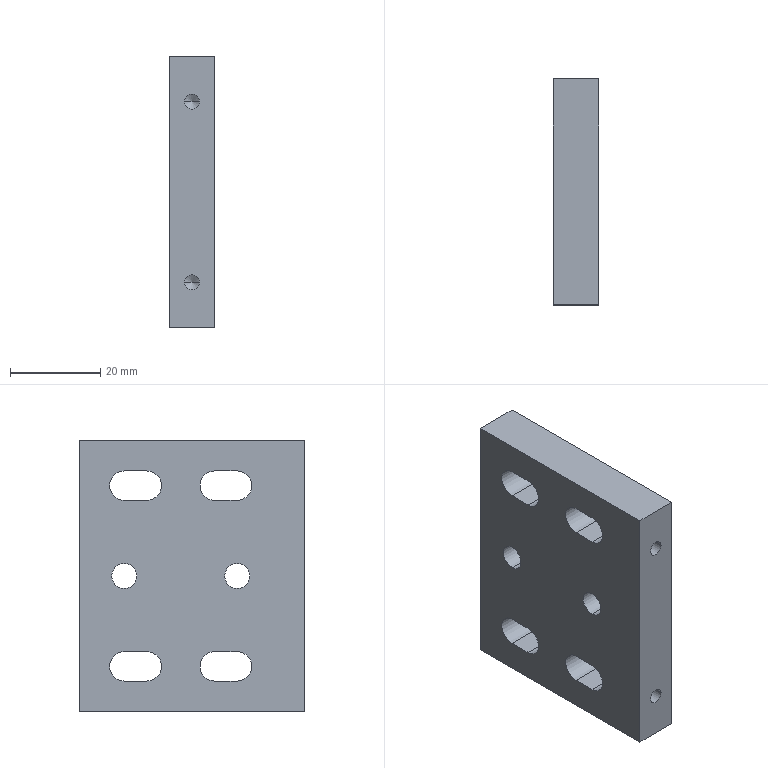Part | STEP file | 09-37 Support plate base | 1 solid | 44 faces | box 10 x 50 x 60 mm | volume 26116 mm3 | cylinder 24 | plane 16 | cone 4 | commonest cylinder face diameters 6.5 x12 3.3 x4 5.5 x4 10 x4